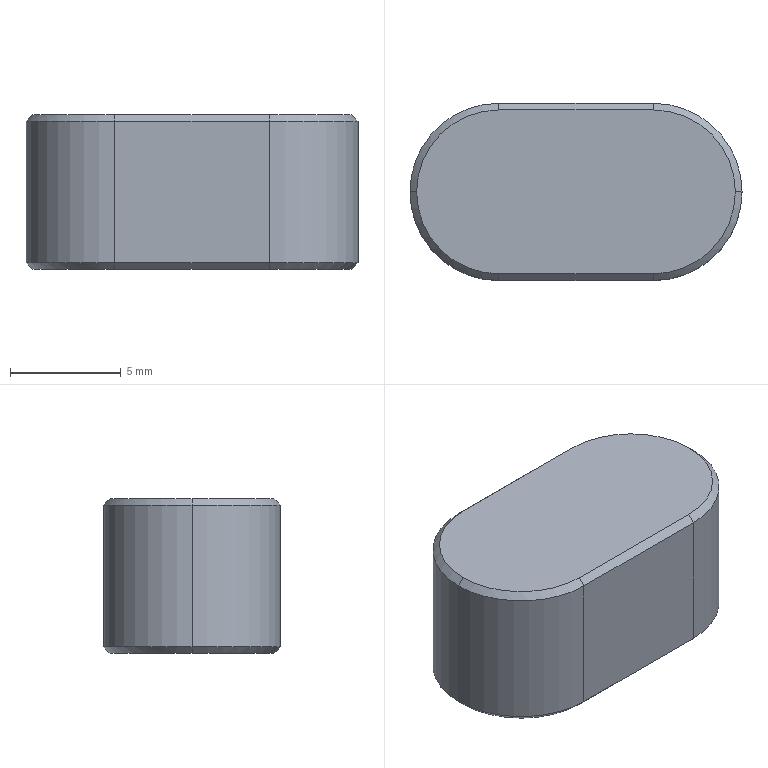Part | SolidWorks | features Chamfer 1, Extrusion 1, Fillet 1 | 1 solid | 20 faces | box 15 x 8 x 7 mm | volume 740.393 mm3 | plane 8 | cone 8 | cylinder 4 | commonest cylinder face diameters 8 x4
STEP:
#1=CARTESIAN_POINT('',(3.5,4.,6.7));
#2=VERTEX_POINT('',#1);
#3=CARTESIAN_POINT('',(3.5,4.,0.3));
#4=VERTEX_POINT('',#3);
#5=CARTESIAN_POINT('',(3.5,4.,7.));
#6=DIRECTION('',(0.,0.,-1.));
#7=VECTOR('',#6,1000.);
#8=LINE('',#5,#7);
#9=EDGE_CURVE('',#2,#4,#8,.T.);
#10=ORIENTED_EDGE('',*,*,#9,.T.);
#11=CARTESIAN_POINT('',(-3.5,4.,0.3));
#12=VERTEX_POINT('',#11);
#13=CARTESIAN_POINT('',(-7.5,4.,0.3));
#14=DIRECTION('',(-1.,0.,0.));
#15=VECTOR('',#14,1000.);
#16=LINE('',#13,#15);
#17=EDGE_CURVE('',#4,#12,#16,.T.);
#18=ORIENTED_EDGE('',*,*,#17,.T.);
#19=CARTESIAN_POINT('',(-3.5,4.,6.7));
#20=VERTEX_POINT('',#19);
#21=CARTESIAN_POINT('',(-3.5,4.,7.));
#22=DIRECTION('',(0.,0.,1.));
#23=VECTOR('',#22,1000.);
#24=LINE('',#21,#23);
#25=EDGE_CURVE('',#12,#20,#24,.T.);
#26=ORIENTED_EDGE('',*,*,#25,.T.);
#27=CARTESIAN_POINT('',(3.5,4.,6.7));
#28=DIRECTION('',(1.,0.,0.));
#29=VECTOR('',#28,1000.);
#30=LINE('',#27,#29);
#31=EDGE_CURVE('',#20,#2,#30,.T.);
#32=ORIENTED_EDGE('',*,*,#31,.T.);
#33=EDGE_LOOP('',(#10,#18,#26,#32));
#34=FACE_OUTER_BOUND('',#33,.T.);
#35=CARTESIAN_POINT('',(-7.5,4.,7.));
#36=DIRECTION('',(0.,-1.,0.));
#37=DIRECTION('',(0.,0.,-1.));
#38=AXIS2_PLACEMENT_3D('',#35,#36,#37);
#39=PLANE('',#38);
#40=ADVANCED_FACE('',(#34),#39,.F.);
#41=CARTESIAN_POINT('',(-3.5,-4.,6.7));
#42=VERTEX_POINT('',#41);
#43=CARTESIAN_POINT('',(-3.5,-4.,0.3));
#44=VERTEX_POINT('',#43);
#45=CARTESIAN_POINT('',(-3.5,-4.,7.));
#46=DIRECTION('',(0.,0.,-1.));
#47=VECTOR('',#46,1000.);
#48=LINE('',#45,#47);
#49=EDGE_CURVE('',#42,#44,#48,.T.);
#50=ORIENTED_EDGE('',*,*,#49,.T.);
#51=CARTESIAN_POINT('',(3.5,-4.,0.3));
#52=VERTEX_POINT('',#51);
#53=CARTESIAN_POINT('',(-7.5,-4.,0.3));
#54=DIRECTION('',(1.,0.,0.));
#55=VECTOR('',#54,1000.);
#56=LINE('',#53,#55);
#57=EDGE_CURVE('',#44,#52,#56,.T.);
#58=ORIENTED_EDGE('',*,*,#57,.T.);
#59=CARTESIAN_POINT('',(3.5,-4.,6.7));
#60=VERTEX_POINT('',#59);
#61=CARTESIAN_POINT('',(3.5,-4.,7.));
#62=DIRECTION('',(0.,0.,1.));
#63=VECTOR('',#62,1000.);
#64=LINE('',#61,#63);
#65=EDGE_CURVE('',#52,#60,#64,.T.);
#66=ORIENTED_EDGE('',*,*,#65,.T.);
#67=CARTESIAN_POINT('',(-3.5,-4.,6.7));
#68=DIRECTION('',(-1.,0.,0.));
#69=VECTOR('',#68,1000.);
#70=LINE('',#67,#69);
#71=EDGE_CURVE('',#60,#42,#70,.T.);
#72=ORIENTED_EDGE('',*,*,#71,.T.);
#73=EDGE_LOOP('',(#50,#58,#66,#72));
#74=FACE_OUTER_BOUND('',#73,.T.);
#75=CARTESIAN_POINT('',(-7.5,-4.,7.));
#76=DIRECTION('',(0.,1.,0.));
#77=DIRECTION('',(0.,0.,1.));
#78=AXIS2_PLACEMENT_3D('',#75,#76,#77);
#79=PLANE('',#78);
#80=ADVANCED_FACE('',(#74),#79,.F.);
#81=CARTESIAN_POINT('',(-7.2,0.,7.));
#82=VERTEX_POINT('',#81);
#83=CARTESIAN_POINT('',(-3.5,-3.7,7.));
#84=VERTEX_POINT('',#83);
#85=CARTESIAN_POINT('',(-3.5,0.,7.));
#86=DIRECTION('',(0.,0.,1.));
#87=DIRECTION('',(1.,0.,0.));
#88=AXIS2_PLACEMENT_3D('',#85,#86,#87);
#89=CIRCLE('',#88,3.7);
#90=EDGE_CURVE('',#82,#84,#89,.T.);
#91=ORIENTED_EDGE('',*,*,#90,.T.);
#92=CARTESIAN_POINT('',(3.5,-3.7,7.));
#93=VERTEX_POINT('',#92);
#94=CARTESIAN_POINT('',(3.5,-3.7,7.));
#95=DIRECTION('',(1.,0.,0.));
#96=VECTOR('',#95,1000.);
#97=LINE('',#94,#96);
#98=EDGE_CURVE('',#84,#93,#97,.T.);
#99=ORIENTED_EDGE('',*,*,#98,.T.);
#100=CARTESIAN_POINT('',(7.2,0.,7.));
#101=VERTEX_POINT('',#100);
#102=CARTESIAN_POINT('',(3.5,0.,7.));
#103=DIRECTION('',(0.,0.,1.));
#104=DIRECTION('',(1.,0.,0.));
#105=AXIS2_PLACEMENT_3D('',#102,#103,#104);
#106=CIRCLE('',#105,3.7);
#107=EDGE_CURVE('',#93,#101,#106,.T.);
#108=ORIENTED_EDGE('',*,*,#107,.T.);
#109=CARTESIAN_POINT('',(3.5,3.7,7.));
#110=VERTEX_POINT('',#109);
#111=CARTESIAN_POINT('',(3.5,0.,7.));
#112=DIRECTION('',(0.,0.,1.));
#113=DIRECTION('',(1.,0.,0.));
#114=AXIS2_PLACEMENT_3D('',#111,#112,#113);
#115=CIRCLE('',#114,3.7);
#116=EDGE_CURVE('',#101,#110,#115,.T.);
#117=ORIENTED_EDGE('',*,*,#116,.T.);
#118=CARTESIAN_POINT('',(-3.5,3.7,7.));
#119=VERTEX_POINT('',#118);
#120=CARTESIAN_POINT('',(-3.5,3.7,7.));
#121=DIRECTION('',(-1.,0.,0.));
#122=VECTOR('',#121,1000.);
#123=LINE('',#120,#122);
#124=EDGE_CURVE('',#110,#119,#123,.T.);
#125=ORIENTED_EDGE('',*,*,#124,.T.);
#126=CARTESIAN_POINT('',(-3.5,0.,7.));
#127=DIRECTION('',(0.,0.,1.));
#128=DIRECTION('',(1.,0.,0.));
#129=AXIS2_PLACEMENT_3D('',#126,#127,#128);
#130=CIRCLE('',#129,3.7);
#131=EDGE_CURVE('',#119,#82,#130,.T.);
#132=ORIENTED_EDGE('',*,*,#131,.T.);
#133=EDGE_LOOP('',(#91,#99,#108,#117,#125,#132));
#134=FACE_OUTER_BOUND('',#133,.T.);
#135=CARTESIAN_POINT('',(0.,0.,7.));
#136=DIRECTION('',(0.,0.,1.));
#137=DIRECTION('',(1.,0.,0.));
#138=AXIS2_PLACEMENT_3D('',#135,#136,#137);
#139=PLANE('',#138);
#140=ADVANCED_FACE('',(#134),#139,.T.);
#141=CARTESIAN_POINT('',(-3.5,-3.7,0.));
#142=VERTEX_POINT('',#141);
#143=CARTESIAN_POINT('',(-7.2,0.,0.));
#144=VERTEX_POINT('',#143);
#145=CARTESIAN_POINT('',(-3.5,0.,0.));
#146=DIRECTION('',(0.,0.,-1.));
#147=DIRECTION('',(1.,0.,0.));
#148=AXIS2_PLACEMENT_3D('',#145,#146,#147);
#149=CIRCLE('',#148,3.7);
#150=EDGE_CURVE('',#142,#144,#149,.T.);
#151=ORIENTED_EDGE('',*,*,#150,.T.);
#152=CARTESIAN_POINT('',(-3.5,3.7,0.));
#153=VERTEX_POINT('',#152);
#154=CARTESIAN_POINT('',(-3.5,0.,0.));
#155=DIRECTION('',(0.,0.,-1.));
#156=DIRECTION('',(1.,0.,0.));
#157=AXIS2_PLACEMENT_3D('',#154,#155,#156);
#158=CIRCLE('',#157,3.7);
#159=EDGE_CURVE('',#144,#153,#158,.T.);
#160=ORIENTED_EDGE('',*,*,#159,.T.);
#161=CARTESIAN_POINT('',(3.5,3.7,0.));
#162=VERTEX_POINT('',#161);
#163=CARTESIAN_POINT('',(0.,3.7,0.));
#164=DIRECTION('',(1.,0.,0.));
#165=VECTOR('',#164,1000.);
#166=LINE('',#163,#165);
#167=EDGE_CURVE('',#153,#162,#166,.T.);
#168=ORIENTED_EDGE('',*,*,#167,.T.);
#169=CARTESIAN_POINT('',(7.2,0.,0.));
#170=VERTEX_POINT('',#169);
#171=CARTESIAN_POINT('',(3.5,0.,0.));
#172=DIRECTION('',(0.,0.,-1.));
#173=DIRECTION('',(1.,0.,0.));
#174=AXIS2_PLACEMENT_3D('',#171,#172,#173);
#175=CIRCLE('',#174,3.7);
#176=EDGE_CURVE('',#162,#170,#175,.T.);
#177=ORIENTED_EDGE('',*,*,#176,.T.);
#178=CARTESIAN_POINT('',(3.5,-3.7,0.));
#179=VERTEX_POINT('',#178);
#180=CARTESIAN_POINT('',(3.5,0.,0.));
#181=DIRECTION('',(0.,0.,-1.));
#182=DIRECTION('',(1.,0.,0.));
#183=AXIS2_PLACEMENT_3D('',#180,#181,#182);
#184=CIRCLE('',#183,3.7);
#185=EDGE_CURVE('',#170,#179,#184,.T.);
#186=ORIENTED_EDGE('',*,*,#185,.T.);
#187=CARTESIAN_POINT('',(0.,-3.7,0.));
#188=DIRECTION('',(-1.,0.,0.));
#189=VECTOR('',#188,1000.);
#190=LINE('',#187,#189);
#191=EDGE_CURVE('',#179,#142,#190,.T.);
#192=ORIENTED_EDGE('',*,*,#191,.T.);
#193=EDGE_LOOP('',(#151,#160,#168,#177,#186,#192));
#194=FACE_OUTER_BOUND('',#193,.T.);
#195=CARTESIAN_POINT('',(0.,0.,0.));
#196=DIRECTION('',(0.,0.,1.));
#197=DIRECTION('',(1.,0.,0.));
#198=AXIS2_PLACEMENT_3D('',#195,#196,#197);
#199=PLANE('',#198);
#200=ADVANCED_FACE('',(#194),#199,.F.);
#201=ORIENTED_EDGE('',*,*,#65,.F.);
#202=CARTESIAN_POINT('',(7.5,0.,0.3));
#203=VERTEX_POINT('',#202);
#204=CARTESIAN_POINT('',(3.5,0.,0.3));
#205=DIRECTION('',(0.,0.,1.));
#206=DIRECTION('',(1.,0.,0.));
#207=AXIS2_PLACEMENT_3D('',#204,#205,#206);
#208=CIRCLE('',#207,4.);
#209=EDGE_CURVE('',#52,#203,#208,.T.);
#210=ORIENTED_EDGE('',*,*,#209,.T.);
#211=CARTESIAN_POINT('',(7.5,0.,6.7));
#212=VERTEX_POINT('',#211);
#213=CARTESIAN_POINT('',(7.5,0.,7.));
#214=DIRECTION('',(0.,0.,-1.));
#215=VECTOR('',#214,1000.);
#216=LINE('',#213,#215);
#217=EDGE_CURVE('',#212,#203,#216,.T.);
#218=ORIENTED_EDGE('',*,*,#217,.F.);
#219=CARTESIAN_POINT('',(3.5,0.,6.7));
#220=DIRECTION('',(0.,0.,-1.));
#221=DIRECTION('',(1.,0.,0.));
#222=AXIS2_PLACEMENT_3D('',#219,#220,#221);
#223=CIRCLE('',#222,4.);
#224=EDGE_CURVE('',#212,#60,#223,.T.);
#225=ORIENTED_EDGE('',*,*,#224,.T.);
#226=EDGE_LOOP('',(#201,#210,#218,#225));
#227=FACE_OUTER_BOUND('',#226,.T.);
#228=CARTESIAN_POINT('',(3.5,0.,7.));
#229=DIRECTION('',(0.,0.,-1.));
#230=DIRECTION('',(-1.,0.,0.));
#231=AXIS2_PLACEMENT_3D('',#228,#229,#230);
#232=CYLINDRICAL_SURFACE('',#231,4.);
#233=ADVANCED_FACE('',(#227),#232,.T.);
#234=ORIENTED_EDGE('',*,*,#217,.T.);
#235=CARTESIAN_POINT('',(3.5,0.,0.3));
#236=DIRECTION('',(0.,0.,1.));
#237=DIRECTION('',(1.,0.,0.));
#238=AXIS2_PLACEMENT_3D('',#235,#236,#237);
#239=CIRCLE('',#238,4.);
#240=EDGE_CURVE('',#203,#4,#239,.T.);
#241=ORIENTED_EDGE('',*,*,#240,.T.);
#242=ORIENTED_EDGE('',*,*,#9,.F.);
#243=CARTESIAN_POINT('',(3.5,0.,6.7));
#244=DIRECTION('',(0.,0.,-1.));
#245=DIRECTION('',(1.,0.,0.));
#246=AXIS2_PLACEMENT_3D('',#243,#244,#245);
#247=CIRCLE('',#246,4.);
#248=EDGE_CURVE('',#2,#212,#247,.T.);
#249=ORIENTED_EDGE('',*,*,#248,.T.);
#250=EDGE_LOOP('',(#234,#241,#242,#249));
#251=FACE_OUTER_BOUND('',#250,.T.);
#252=CARTESIAN_POINT('',(3.5,0.,7.));
#253=DIRECTION('',(0.,0.,-1.));
#254=DIRECTION('',(-1.,0.,0.));
#255=AXIS2_PLACEMENT_3D('',#252,#253,#254);
#256=CYLINDRICAL_SURFACE('',#255,4.);
#257=ADVANCED_FACE('',(#251),#256,.T.);
#258=CARTESIAN_POINT('',(-7.5,0.,0.3));
#259=VERTEX_POINT('',#258);
#260=CARTESIAN_POINT('',(-7.5,0.,6.7));
#261=VERTEX_POINT('',#260);
#262=CARTESIAN_POINT('',(-7.5,0.,7.));
#263=DIRECTION('',(0.,0.,1.));
#264=VECTOR('',#263,1000.);
#265=LINE('',#262,#264);
#266=EDGE_CURVE('',#259,#261,#265,.T.);
#267=ORIENTED_EDGE('',*,*,#266,.F.);
#268=CARTESIAN_POINT('',(-3.5,0.,0.3));
#269=DIRECTION('',(0.,0.,1.));
#270=DIRECTION('',(1.,0.,0.));
#271=AXIS2_PLACEMENT_3D('',#268,#269,#270);
#272=CIRCLE('',#271,4.);
#273=EDGE_CURVE('',#259,#44,#272,.T.);
#274=ORIENTED_EDGE('',*,*,#273,.T.);
#275=ORIENTED_EDGE('',*,*,#49,.F.);
#276=CARTESIAN_POINT('',(-3.5,0.,6.7));
#277=DIRECTION('',(0.,0.,-1.));
#278=DIRECTION('',(1.,0.,0.));
#279=AXIS2_PLACEMENT_3D('',#276,#277,#278);
#280=CIRCLE('',#279,4.);
#281=EDGE_CURVE('',#42,#261,#280,.T.);
#282=ORIENTED_EDGE('',*,*,#281,.T.);
#283=EDGE_LOOP('',(#267,#274,#275,#282));
#284=FACE_OUTER_BOUND('',#283,.T.);
#285=CARTESIAN_POINT('',(-3.5,0.,7.));
#286=DIRECTION('',(0.,0.,-1.));
#287=DIRECTION('',(-1.,0.,0.));
#288=AXIS2_PLACEMENT_3D('',#285,#286,#287);
#289=CYLINDRICAL_SURFACE('',#288,4.);
#290=ADVANCED_FACE('',(#284),#289,.T.);
#291=ORIENTED_EDGE('',*,*,#25,.F.);
#292=CARTESIAN_POINT('',(-3.5,0.,0.3));
#293=DIRECTION('',(0.,0.,1.));
#294=DIRECTION('',(1.,0.,0.));
#295=AXIS2_PLACEMENT_3D('',#292,#293,#294);
#296=CIRCLE('',#295,4.);
#297=EDGE_CURVE('',#12,#259,#296,.T.);
#298=ORIENTED_EDGE('',*,*,#297,.T.);
#299=ORIENTED_EDGE('',*,*,#266,.T.);
#300=CARTESIAN_POINT('',(-3.5,0.,6.7));
#301=DIRECTION('',(0.,0.,-1.));
#302=DIRECTION('',(1.,0.,0.));
#303=AXIS2_PLACEMENT_3D('',#300,#301,#302);
#304=CIRCLE('',#303,4.);
#305=EDGE_CURVE('',#261,#20,#304,.T.);
#306=ORIENTED_EDGE('',*,*,#305,.T.);
#307=EDGE_LOOP('',(#291,#298,#299,#306));
#308=FACE_OUTER_BOUND('',#307,.T.);
#309=CARTESIAN_POINT('',(-3.5,0.,7.));
#310=DIRECTION('',(0.,0.,-1.));
#311=DIRECTION('',(-1.,0.,0.));
#312=AXIS2_PLACEMENT_3D('',#309,#310,#311);
#313=CYLINDRICAL_SURFACE('',#312,4.);
#314=ADVANCED_FACE('',(#308),#313,.T.);
#315=CARTESIAN_POINT('',(7.5,0.,0.3));
#316=DIRECTION('',(-0.7071,0.,-0.7071));
#317=VECTOR('',#316,1000.);
#318=LINE('',#315,#317);
#319=EDGE_CURVE('',#203,#170,#318,.T.);
#320=ORIENTED_EDGE('',*,*,#319,.F.);
#321=ORIENTED_EDGE('',*,*,#209,.F.);
#322=CARTESIAN_POINT('',(3.5,-3.7,0.));
#323=DIRECTION('',(0.,-0.7071,0.7071));
#324=VECTOR('',#323,1000.);
#325=LINE('',#322,#324);
#326=EDGE_CURVE('',#179,#52,#325,.T.);
#327=ORIENTED_EDGE('',*,*,#326,.F.);
#328=ORIENTED_EDGE('',*,*,#185,.F.);
#329=EDGE_LOOP('',(#320,#321,#327,#328));
#330=FACE_OUTER_BOUND('',#329,.T.);
#331=CARTESIAN_POINT('',(3.5,0.,0.));
#332=DIRECTION('',(0.,0.,1.));
#333=DIRECTION('',(1.,0.,0.));
#334=AXIS2_PLACEMENT_3D('',#331,#332,#333);
#335=CONICAL_SURFACE('',#334,3.7,0.7854);
#336=ADVANCED_FACE('',(#330),#335,.T.);
#337=ORIENTED_EDGE('',*,*,#326,.T.);
#338=ORIENTED_EDGE('',*,*,#57,.F.);
#339=CARTESIAN_POINT('',(-3.5,-3.7,0.));
#340=DIRECTION('',(0.,-0.7071,0.7071));
#341=VECTOR('',#340,1000.);
#342=LINE('',#339,#341);
#343=EDGE_CURVE('',#142,#44,#342,.T.);
#344=ORIENTED_EDGE('',*,*,#343,.F.);
#345=ORIENTED_EDGE('',*,*,#191,.F.);
#346=EDGE_LOOP('',(#337,#338,#344,#345));
#347=FACE_OUTER_BOUND('',#346,.T.);
#348=CARTESIAN_POINT('',(-7.5,-4.,0.3));
#349=DIRECTION('',(0.,0.7071,0.7071));
#350=DIRECTION('',(1.,0.,0.));
#351=AXIS2_PLACEMENT_3D('',#348,#349,#350);
#352=PLANE('',#351);
#353=ADVANCED_FACE('',(#347),#352,.F.);
#354=ORIENTED_EDGE('',*,*,#319,.T.);
#355=ORIENTED_EDGE('',*,*,#176,.F.);
#356=CARTESIAN_POINT('',(3.5,4.,0.3));
#357=DIRECTION('',(0.,-0.7071,-0.7071));
#358=VECTOR('',#357,1000.);
#359=LINE('',#356,#358);
#360=EDGE_CURVE('',#4,#162,#359,.T.);
#361=ORIENTED_EDGE('',*,*,#360,.F.);
#362=ORIENTED_EDGE('',*,*,#240,.F.);
#363=EDGE_LOOP('',(#354,#355,#361,#362));
#364=FACE_OUTER_BOUND('',#363,.T.);
#365=CARTESIAN_POINT('',(3.5,0.,0.));
#366=DIRECTION('',(0.,0.,1.));
#367=DIRECTION('',(1.,0.,0.));
#368=AXIS2_PLACEMENT_3D('',#365,#366,#367);
#369=CONICAL_SURFACE('',#368,3.7,0.7854);
#370=ADVANCED_FACE('',(#364),#369,.T.);
#371=ORIENTED_EDGE('',*,*,#343,.T.);
#372=ORIENTED_EDGE('',*,*,#273,.F.);
#373=CARTESIAN_POINT('',(-7.2,0.,0.));
#374=DIRECTION('',(-0.7071,0.,0.7071));
#375=VECTOR('',#374,1000.);
#376=LINE('',#373,#375);
#377=EDGE_CURVE('',#144,#259,#376,.T.);
#378=ORIENTED_EDGE('',*,*,#377,.F.);
#379=ORIENTED_EDGE('',*,*,#150,.F.);
#380=EDGE_LOOP('',(#371,#372,#378,#379));
#381=FACE_OUTER_BOUND('',#380,.T.);
#382=CARTESIAN_POINT('',(-3.5,0.,0.));
#383=DIRECTION('',(0.,0.,1.));
#384=DIRECTION('',(1.,0.,0.));
#385=AXIS2_PLACEMENT_3D('',#382,#383,#384);
#386=CONICAL_SURFACE('',#385,3.7,0.7854);
#387=ADVANCED_FACE('',(#381),#386,.T.);
#388=ORIENTED_EDGE('',*,*,#360,.T.);
#389=ORIENTED_EDGE('',*,*,#167,.F.);
#390=CARTESIAN_POINT('',(-3.5,4.,0.3));
#391=DIRECTION('',(0.,-0.7071,-0.7071));
#392=VECTOR('',#391,1000.);
#393=LINE('',#390,#392);
#394=EDGE_CURVE('',#12,#153,#393,.T.);
#395=ORIENTED_EDGE('',*,*,#394,.F.);
#396=ORIENTED_EDGE('',*,*,#17,.F.);
#397=EDGE_LOOP('',(#388,#389,#395,#396));
#398=FACE_OUTER_BOUND('',#397,.T.);
#399=CARTESIAN_POINT('',(-7.5,4.,0.3));
#400=DIRECTION('',(0.,-0.7071,0.7071));
#401=DIRECTION('',(-1.,0.,0.));
#402=AXIS2_PLACEMENT_3D('',#399,#400,#401);
#403=PLANE('',#402);
#404=ADVANCED_FACE('',(#398),#403,.F.);
#405=ORIENTED_EDGE('',*,*,#377,.T.);
#406=ORIENTED_EDGE('',*,*,#297,.F.);
#407=ORIENTED_EDGE('',*,*,#394,.T.);
#408=ORIENTED_EDGE('',*,*,#159,.F.);
#409=EDGE_LOOP('',(#405,#406,#407,#408));
#410=FACE_OUTER_BOUND('',#409,.T.);
#411=CARTESIAN_POINT('',(-3.5,0.,0.));
#412=DIRECTION('',(0.,0.,1.));
#413=DIRECTION('',(1.,0.,0.));
#414=AXIS2_PLACEMENT_3D('',#411,#412,#413);
#415=CONICAL_SURFACE('',#414,3.7,0.7854);
#416=ADVANCED_FACE('',(#410),#415,.T.);
#417=CARTESIAN_POINT('',(3.5,4.,6.7));
#418=DIRECTION('',(0.,-0.7071,0.7071));
#419=VECTOR('',#418,1000.);
#420=LINE('',#417,#419);
#421=EDGE_CURVE('',#2,#110,#420,.T.);
#422=ORIENTED_EDGE('',*,*,#421,.F.);
#423=ORIENTED_EDGE('',*,*,#31,.F.);
#424=CARTESIAN_POINT('',(-3.5,3.7,7.));
#425=DIRECTION('',(0.,0.7071,-0.7071));
#426=VECTOR('',#425,1000.);
#427=LINE('',#424,#426);
#428=EDGE_CURVE('',#119,#20,#427,.T.);
#429=ORIENTED_EDGE('',*,*,#428,.F.);
#430=ORIENTED_EDGE('',*,*,#124,.F.);
#431=EDGE_LOOP('',(#422,#423,#429,#430));
#432=FACE_OUTER_BOUND('',#431,.T.);
#433=CARTESIAN_POINT('',(0.,3.7,7.));
#434=DIRECTION('',(0.,0.7071,0.7071));
#435=DIRECTION('',(1.,0.,0.));
#436=AXIS2_PLACEMENT_3D('',#433,#434,#435);
#437=PLANE('',#436);
#438=ADVANCED_FACE('',(#432),#437,.T.);
#439=ORIENTED_EDGE('',*,*,#428,.T.);
#440=ORIENTED_EDGE('',*,*,#305,.F.);
#441=CARTESIAN_POINT('',(-7.2,0.,7.));
#442=DIRECTION('',(-0.7071,0.,-0.7071));
#443=VECTOR('',#442,1000.);
#444=LINE('',#441,#443);
#445=EDGE_CURVE('',#82,#261,#444,.T.);
#446=ORIENTED_EDGE('',*,*,#445,.F.);
#447=ORIENTED_EDGE('',*,*,#131,.F.);
#448=EDGE_LOOP('',(#439,#440,#446,#447));
#449=FACE_OUTER_BOUND('',#448,.T.);
#450=CARTESIAN_POINT('',(-3.5,0.,7.));
#451=DIRECTION('',(0.,0.,-1.));
#452=DIRECTION('',(-1.,0.,0.));
#453=AXIS2_PLACEMENT_3D('',#450,#451,#452);
#454=CONICAL_SURFACE('',#453,3.7,0.7854);
#455=ADVANCED_FACE('',(#449),#454,.T.);
#456=ORIENTED_EDGE('',*,*,#421,.T.);
#457=ORIENTED_EDGE('',*,*,#116,.F.);
#458=CARTESIAN_POINT('',(7.5,0.,6.7));
#459=DIRECTION('',(-0.7071,0.,0.7071));
#460=VECTOR('',#459,1000.);
#461=LINE('',#458,#460);
#462=EDGE_CURVE('',#212,#101,#461,.T.);
#463=ORIENTED_EDGE('',*,*,#462,.F.);
#464=ORIENTED_EDGE('',*,*,#248,.F.);
#465=EDGE_LOOP('',(#456,#457,#463,#464));
#466=FACE_OUTER_BOUND('',#465,.T.);
#467=CARTESIAN_POINT('',(3.5,0.,7.));
#468=DIRECTION('',(0.,0.,-1.));
#469=DIRECTION('',(-1.,0.,0.));
#470=AXIS2_PLACEMENT_3D('',#467,#468,#469);
#471=CONICAL_SURFACE('',#470,3.7,0.7854);
#472=ADVANCED_FACE('',(#466),#471,.T.);
#473=ORIENTED_EDGE('',*,*,#445,.T.);
#474=ORIENTED_EDGE('',*,*,#281,.F.);
#475=CARTESIAN_POINT('',(-3.5,-3.7,7.));
#476=DIRECTION('',(0.,-0.7071,-0.7071));
#477=VECTOR('',#476,1000.);
#478=LINE('',#475,#477);
#479=EDGE_CURVE('',#84,#42,#478,.T.);
#480=ORIENTED_EDGE('',*,*,#479,.F.);
#481=ORIENTED_EDGE('',*,*,#90,.F.);
#482=EDGE_LOOP('',(#473,#474,#480,#481));
#483=FACE_OUTER_BOUND('',#482,.T.);
#484=CARTESIAN_POINT('',(-3.5,0.,7.));
#485=DIRECTION('',(0.,0.,-1.));
#486=DIRECTION('',(-1.,0.,0.));
#487=AXIS2_PLACEMENT_3D('',#484,#485,#486);
#488=CONICAL_SURFACE('',#487,3.7,0.7854);
#489=ADVANCED_FACE('',(#483),#488,.T.);
#490=ORIENTED_EDGE('',*,*,#462,.T.);
#491=ORIENTED_EDGE('',*,*,#107,.F.);
#492=CARTESIAN_POINT('',(3.5,-4.,6.7));
#493=DIRECTION('',(0.,0.7071,0.7071));
#494=VECTOR('',#493,1000.);
#495=LINE('',#492,#494);
#496=EDGE_CURVE('',#60,#93,#495,.T.);
#497=ORIENTED_EDGE('',*,*,#496,.F.);
#498=ORIENTED_EDGE('',*,*,#224,.F.);
#499=EDGE_LOOP('',(#490,#491,#497,#498));
#500=FACE_OUTER_BOUND('',#499,.T.);
#501=CARTESIAN_POINT('',(3.5,0.,7.));
#502=DIRECTION('',(0.,0.,-1.));
#503=DIRECTION('',(-1.,0.,0.));
#504=AXIS2_PLACEMENT_3D('',#501,#502,#503);
#505=CONICAL_SURFACE('',#504,3.7,0.7854);
#506=ADVANCED_FACE('',(#500),#505,.T.);
#507=ORIENTED_EDGE('',*,*,#479,.T.);
#508=ORIENTED_EDGE('',*,*,#71,.F.);
#509=ORIENTED_EDGE('',*,*,#496,.T.);
#510=ORIENTED_EDGE('',*,*,#98,.F.);
#511=EDGE_LOOP('',(#507,#508,#509,#510));
#512=FACE_OUTER_BOUND('',#511,.T.);
#513=CARTESIAN_POINT('',(0.,-3.7,7.));
#514=DIRECTION('',(0.,-0.7071,0.7071));
#515=DIRECTION('',(-1.,0.,0.));
#516=AXIS2_PLACEMENT_3D('',#513,#514,#515);
#517=PLANE('',#516);
#518=ADVANCED_FACE('',(#512),#517,.T.);
#519=CLOSED_SHELL('',(#40,#80,#140,#200,#233,#257,#290,#314,#336,#353,#370,#387,#404,#416,#438,#455,#472,#489,#506,#518));
#520=MANIFOLD_SOLID_BREP('',#519);
#521=CARTESIAN_POINT('',(0.,0.,0.));
#522=DIRECTION('',(0.,0.,1.));
#523=DIRECTION('',(1.,0.,0.));
#524=AXIS2_PLACEMENT_3D('',#521,#522,#523);
#525=(LENGTH_UNIT()NAMED_UNIT(*)SI_UNIT(.MILLI.,.METRE.));
#526=UNCERTAINTY_MEASURE_WITH_UNIT(LENGTH_MEASURE(0.00001),#525,'','');
#527=(NAMED_UNIT(*)PLANE_ANGLE_UNIT()SI_UNIT($,.RADIAN.));
#528=(NAMED_UNIT(*)SI_UNIT($,.STERADIAN.)SOLID_ANGLE_UNIT());
#529=(GEOMETRIC_REPRESENTATION_CONTEXT(3)GLOBAL_UNCERTAINTY_ASSIGNED_CONTEXT((#526))GLOBAL_UNIT_ASSIGNED_CONTEXT((#525,#527,#528))REPRESENTATION_CONTEXT('',''));
#530=ADVANCED_BREP_SHAPE_REPRESENTATION('',(#520,#524),#529);